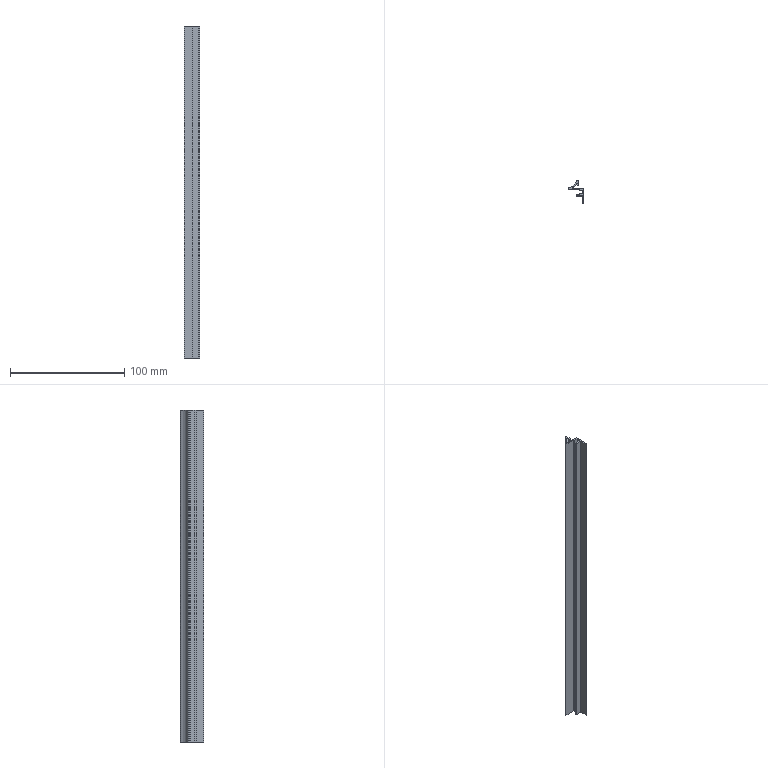Part | SolidWorks | features MoveFace 2, BaseBody 1, ICE 1 | 1 solid | 27 faces | box 14 x 20.3 x 291 mm | volume 14816 mm3 | plane 20 | cylinder 7 | commonest cylinder face diameters 0.387 x2 0.8 x2 0.4 x1 20 x1 22 x1
STEP:
#1=CARTESIAN_POINT('',(-5.304,-0.625,-867.));
#2=VERTEX_POINT('',#1);
#3=CARTESIAN_POINT('',(-5.449,-0.8125,-867.));
#4=VERTEX_POINT('',#3);
#5=CARTESIAN_POINT('',(-5.255,-0.8125,-867.));
#6=DIRECTION('',(0.,0.,1.));
#7=DIRECTION('',(-1.,0.,0.));
#8=AXIS2_PLACEMENT_3D('',#5,#6,#7);
#9=CIRCLE('',#8,0.1937);
#10=EDGE_CURVE('',#2,#4,#9,.T.);
#11=ORIENTED_EDGE('',*,*,#10,.T.);
#12=CARTESIAN_POINT('',(-5.449,-0.8125,-1158.));
#13=VERTEX_POINT('',#12);
#14=CARTESIAN_POINT('',(-5.449,-0.8125,230.));
#15=DIRECTION('',(0.,0.,-1.));
#16=VECTOR('',#15,1000.);
#17=LINE('',#14,#16);
#18=EDGE_CURVE('',#4,#13,#17,.T.);
#19=ORIENTED_EDGE('',*,*,#18,.T.);
#20=CARTESIAN_POINT('',(-5.304,-0.625,-1158.));
#21=VERTEX_POINT('',#20);
#22=CARTESIAN_POINT('',(-5.255,-0.8125,-1158.));
#23=DIRECTION('',(0.,0.,-1.));
#24=DIRECTION('',(1.,0.,0.));
#25=AXIS2_PLACEMENT_3D('',#22,#23,#24);
#26=CIRCLE('',#25,0.1937);
#27=EDGE_CURVE('',#13,#21,#26,.T.);
#28=ORIENTED_EDGE('',*,*,#27,.T.);
#29=CARTESIAN_POINT('',(-5.304,-0.625,230.));
#30=DIRECTION('',(0.,0.,-1.));
#31=VECTOR('',#30,1000.);
#32=LINE('',#29,#31);
#33=EDGE_CURVE('',#2,#21,#32,.T.);
#34=ORIENTED_EDGE('',*,*,#33,.F.);
#35=EDGE_LOOP('',(#11,#19,#28,#34));
#36=FACE_OUTER_BOUND('',#35,.T.);
#37=CARTESIAN_POINT('',(-5.255,-0.8125,230.));
#38=DIRECTION('',(0.,0.,-1.));
#39=DIRECTION('',(-1.,0.,0.));
#40=AXIS2_PLACEMENT_3D('',#37,#38,#39);
#41=CYLINDRICAL_SURFACE('',#40,0.1937);
#42=ADVANCED_FACE('',(#36),#41,.F.);
#43=CARTESIAN_POINT('',(5.,-1.,-1158.));
#44=VERTEX_POINT('',#43);
#45=CARTESIAN_POINT('',(5.,-14.3,-1158.));
#46=VERTEX_POINT('',#45);
#47=CARTESIAN_POINT('',(5.,29.623,-1158.));
#48=DIRECTION('',(0.,-1.,0.));
#49=VECTOR('',#48,1000.);
#50=LINE('',#47,#49);
#51=EDGE_CURVE('',#44,#46,#50,.T.);
#52=ORIENTED_EDGE('',*,*,#51,.F.);
#53=CARTESIAN_POINT('',(5.,-1.,-867.));
#54=VERTEX_POINT('',#53);
#55=CARTESIAN_POINT('',(5.,-1.,230.));
#56=DIRECTION('',(0.,0.,-1.));
#57=VECTOR('',#56,1000.);
#58=LINE('',#55,#57);
#59=EDGE_CURVE('',#54,#44,#58,.T.);
#60=ORIENTED_EDGE('',*,*,#59,.F.);
#61=CARTESIAN_POINT('',(5.,-14.3,-867.));
#62=VERTEX_POINT('',#61);
#63=CARTESIAN_POINT('',(5.,29.623,-867.));
#64=DIRECTION('',(0.,1.,0.));
#65=VECTOR('',#64,1000.);
#66=LINE('',#63,#65);
#67=EDGE_CURVE('',#62,#54,#66,.T.);
#68=ORIENTED_EDGE('',*,*,#67,.F.);
#69=CARTESIAN_POINT('',(5.,-14.3,230.));
#70=DIRECTION('',(0.,0.,1.));
#71=VECTOR('',#70,1000.);
#72=LINE('',#69,#71);
#73=EDGE_CURVE('',#46,#62,#72,.T.);
#74=ORIENTED_EDGE('',*,*,#73,.F.);
#75=EDGE_LOOP('',(#52,#60,#68,#74));
#76=FACE_OUTER_BOUND('',#75,.T.);
#77=CARTESIAN_POINT('',(5.,-14.3,230.));
#78=DIRECTION('',(-1.,0.,0.));
#79=DIRECTION('',(0.,0.,1.));
#80=AXIS2_PLACEMENT_3D('',#77,#78,#79);
#81=PLANE('',#80);
#82=ADVANCED_FACE('',(#76),#81,.F.);
#83=CARTESIAN_POINT('',(-9.,-2.,-1158.));
#84=VERTEX_POINT('',#83);
#85=CARTESIAN_POINT('',(-9.,-2.,-867.));
#86=VERTEX_POINT('',#85);
#87=CARTESIAN_POINT('',(-9.,-2.,230.));
#88=DIRECTION('',(0.,0.,1.));
#89=VECTOR('',#88,1000.);
#90=LINE('',#87,#89);
#91=EDGE_CURVE('',#84,#86,#90,.T.);
#92=ORIENTED_EDGE('',*,*,#91,.F.);
#93=CARTESIAN_POINT('',(0.9,-2.,-1158.));
#94=VERTEX_POINT('',#93);
#95=CARTESIAN_POINT('',(5.,-2.,-1158.));
#96=DIRECTION('',(-1.,0.,0.));
#97=VECTOR('',#96,1000.);
#98=LINE('',#95,#97);
#99=EDGE_CURVE('',#94,#84,#98,.T.);
#100=ORIENTED_EDGE('',*,*,#99,.F.);
#101=CARTESIAN_POINT('',(0.9,-2.,-867.));
#102=VERTEX_POINT('',#101);
#103=CARTESIAN_POINT('',(0.9,-2.,230.));
#104=DIRECTION('',(0.,0.,-1.));
#105=VECTOR('',#104,1000.);
#106=LINE('',#103,#105);
#107=EDGE_CURVE('',#102,#94,#106,.T.);
#108=ORIENTED_EDGE('',*,*,#107,.F.);
#109=CARTESIAN_POINT('',(5.,-2.,-867.));
#110=DIRECTION('',(1.,0.,0.));
#111=VECTOR('',#110,1000.);
#112=LINE('',#109,#111);
#113=EDGE_CURVE('',#86,#102,#112,.T.);
#114=ORIENTED_EDGE('',*,*,#113,.F.);
#115=EDGE_LOOP('',(#92,#100,#108,#114));
#116=FACE_OUTER_BOUND('',#115,.T.);
#117=CARTESIAN_POINT('',(-9.,-2.,230.));
#118=DIRECTION('',(0.,1.,0.));
#119=DIRECTION('',(0.,0.,1.));
#120=AXIS2_PLACEMENT_3D('',#117,#118,#119);
#121=PLANE('',#120);
#122=ADVANCED_FACE('',(#116),#121,.F.);
#123=CARTESIAN_POINT('',(4.,-6.,-867.));
#124=VERTEX_POINT('',#123);
#125=CARTESIAN_POINT('',(4.,-3.,-867.));
#126=VERTEX_POINT('',#125);
#127=CARTESIAN_POINT('',(4.,-3.,-867.));
#128=DIRECTION('',(0.,1.,0.));
#129=VECTOR('',#128,1000.);
#130=LINE('',#127,#129);
#131=EDGE_CURVE('',#124,#126,#130,.T.);
#132=ORIENTED_EDGE('',*,*,#131,.F.);
#133=CARTESIAN_POINT('',(1.,-6.,-867.));
#134=VERTEX_POINT('',#133);
#135=CARTESIAN_POINT('',(4.,-6.,-867.));
#136=DIRECTION('',(1.,0.,0.));
#137=VECTOR('',#136,1000.);
#138=LINE('',#135,#137);
#139=EDGE_CURVE('',#134,#124,#138,.T.);
#140=ORIENTED_EDGE('',*,*,#139,.F.);
#141=CARTESIAN_POINT('',(1.,-6.7,-867.));
#142=VERTEX_POINT('',#141);
#143=CARTESIAN_POINT('',(1.,29.623,-867.));
#144=DIRECTION('',(0.,-1.,0.));
#145=VECTOR('',#144,1000.);
#146=LINE('',#143,#145);
#147=EDGE_CURVE('',#134,#142,#146,.T.);
#148=ORIENTED_EDGE('',*,*,#147,.T.);
#149=CARTESIAN_POINT('',(-1.7,-6.7,-867.));
#150=VERTEX_POINT('',#149);
#151=CARTESIAN_POINT('',(1.,-6.7,-867.));
#152=DIRECTION('',(1.,0.,0.));
#153=VECTOR('',#152,1000.);
#154=LINE('',#151,#153);
#155=EDGE_CURVE('',#150,#142,#154,.T.);
#156=ORIENTED_EDGE('',*,*,#155,.F.);
#157=CARTESIAN_POINT('',(-1.7,-7.7,-867.));
#158=VERTEX_POINT('',#157);
#159=CARTESIAN_POINT('',(-1.7,29.623,-867.));
#160=DIRECTION('',(0.,-1.,0.));
#161=VECTOR('',#160,1000.);
#162=LINE('',#159,#161);
#163=EDGE_CURVE('',#150,#158,#162,.T.);
#164=ORIENTED_EDGE('',*,*,#163,.T.);
#165=CARTESIAN_POINT('',(4.,-7.7,-867.));
#166=VERTEX_POINT('',#165);
#167=CARTESIAN_POINT('',(-1.7,-7.7,-867.));
#168=DIRECTION('',(-1.,0.,0.));
#169=VECTOR('',#168,1000.);
#170=LINE('',#167,#169);
#171=EDGE_CURVE('',#166,#158,#170,.T.);
#172=ORIENTED_EDGE('',*,*,#171,.F.);
#173=CARTESIAN_POINT('',(4.,-14.3,-867.));
#174=VERTEX_POINT('',#173);
#175=CARTESIAN_POINT('',(4.,-7.7,-867.));
#176=DIRECTION('',(0.,1.,0.));
#177=VECTOR('',#176,1000.);
#178=LINE('',#175,#177);
#179=EDGE_CURVE('',#174,#166,#178,.T.);
#180=ORIENTED_EDGE('',*,*,#179,.F.);
#181=CARTESIAN_POINT('',(4.,-14.3,-867.));
#182=DIRECTION('',(-1.,0.,0.));
#183=VECTOR('',#182,1000.);
#184=LINE('',#181,#183);
#185=EDGE_CURVE('',#62,#174,#184,.T.);
#186=ORIENTED_EDGE('',*,*,#185,.F.);
#187=ORIENTED_EDGE('',*,*,#67,.T.);
#188=CARTESIAN_POINT('',(-5.207,-1.,-867.));
#189=VERTEX_POINT('',#188);
#190=CARTESIAN_POINT('',(5.,-1.,-867.));
#191=DIRECTION('',(1.,0.,0.));
#192=VECTOR('',#191,1000.);
#193=LINE('',#190,#192);
#194=EDGE_CURVE('',#189,#54,#193,.T.);
#195=ORIENTED_EDGE('',*,*,#194,.F.);
#196=CARTESIAN_POINT('',(-5.255,-0.8125,-867.));
#197=DIRECTION('',(0.,0.,1.));
#198=DIRECTION('',(-1.,0.,0.));
#199=AXIS2_PLACEMENT_3D('',#196,#197,#198);
#200=CIRCLE('',#199,0.1937);
#201=EDGE_CURVE('',#4,#189,#200,.T.);
#202=ORIENTED_EDGE('',*,*,#201,.F.);
#203=ORIENTED_EDGE('',*,*,#10,.F.);
#204=CARTESIAN_POINT('',(-1.368,3.063,-867.));
#205=VERTEX_POINT('',#204);
#206=CARTESIAN_POINT('',(-10.628,9.,-867.));
#207=DIRECTION('',(0.,0.,1.));
#208=DIRECTION('',(-1.,0.,0.));
#209=AXIS2_PLACEMENT_3D('',#206,#207,#208);
#210=CIRCLE('',#209,11.);
#211=EDGE_CURVE('',#2,#205,#210,.T.);
#212=ORIENTED_EDGE('',*,*,#211,.T.);
#213=CARTESIAN_POINT('',(-1.,2.955,-867.));
#214=VERTEX_POINT('',#213);
#215=CARTESIAN_POINT('',(-1.2,2.955,-867.));
#216=DIRECTION('',(0.,0.,1.));
#217=DIRECTION('',(-1.,0.,0.));
#218=AXIS2_PLACEMENT_3D('',#215,#216,#217);
#219=CIRCLE('',#218,0.2);
#220=EDGE_CURVE('',#214,#205,#219,.T.);
#221=ORIENTED_EDGE('',*,*,#220,.F.);
#222=CARTESIAN_POINT('',(-1.,1.5,-867.));
#223=VERTEX_POINT('',#222);
#224=CARTESIAN_POINT('',(-1.,2.955,-867.));
#225=DIRECTION('',(0.,1.,0.));
#226=VECTOR('',#225,1000.);
#227=LINE('',#224,#226);
#228=EDGE_CURVE('',#223,#214,#227,.T.);
#229=ORIENTED_EDGE('',*,*,#228,.F.);
#230=CARTESIAN_POINT('',(0.,1.5,-867.));
#231=VERTEX_POINT('',#230);
#232=CARTESIAN_POINT('',(-1.,1.5,-867.));
#233=DIRECTION('',(-1.,0.,0.));
#234=VECTOR('',#233,1000.);
#235=LINE('',#232,#234);
#236=EDGE_CURVE('',#231,#223,#235,.T.);
#237=ORIENTED_EDGE('',*,*,#236,.F.);
#238=CARTESIAN_POINT('',(0.,6.,-867.));
#239=VERTEX_POINT('',#238);
#240=CARTESIAN_POINT('',(0.,1.5,-867.));
#241=DIRECTION('',(0.,-1.,0.));
#242=VECTOR('',#241,1000.);
#243=LINE('',#240,#242);
#244=EDGE_CURVE('',#239,#231,#243,.T.);
#245=ORIENTED_EDGE('',*,*,#244,.F.);
#246=CARTESIAN_POINT('',(-0.8,6.,-867.));
#247=VERTEX_POINT('',#246);
#248=CARTESIAN_POINT('',(0.,6.,-867.));
#249=DIRECTION('',(1.,0.,0.));
#250=VECTOR('',#249,1000.);
#251=LINE('',#248,#250);
#252=EDGE_CURVE('',#247,#239,#251,.T.);
#253=ORIENTED_EDGE('',*,*,#252,.F.);
#254=CARTESIAN_POINT('',(-1.178,5.731,-867.));
#255=VERTEX_POINT('',#254);
#256=CARTESIAN_POINT('',(-0.8,5.6,-867.));
#257=DIRECTION('',(0.,0.,1.));
#258=DIRECTION('',(-1.,0.,0.));
#259=AXIS2_PLACEMENT_3D('',#256,#257,#258);
#260=CIRCLE('',#259,0.4);
#261=EDGE_CURVE('',#247,#255,#260,.T.);
#262=ORIENTED_EDGE('',*,*,#261,.T.);
#263=CARTESIAN_POINT('',(-8.678,-0.8077,-867.));
#264=VERTEX_POINT('',#263);
#265=CARTESIAN_POINT('',(-10.628,9.,-867.));
#266=DIRECTION('',(0.,0.,1.));
#267=DIRECTION('',(-1.,0.,0.));
#268=AXIS2_PLACEMENT_3D('',#265,#266,#267);
#269=CIRCLE('',#268,10.);
#270=EDGE_CURVE('',#264,#255,#269,.T.);
#271=ORIENTED_EDGE('',*,*,#270,.F.);
#272=CARTESIAN_POINT('',(-9.,-1.2,-867.));
#273=VERTEX_POINT('',#272);
#274=CARTESIAN_POINT('',(-8.6,-1.2,-867.));
#275=DIRECTION('',(0.,0.,1.));
#276=DIRECTION('',(-1.,0.,0.));
#277=AXIS2_PLACEMENT_3D('',#274,#275,#276);
#278=CIRCLE('',#277,0.4);
#279=EDGE_CURVE('',#264,#273,#278,.T.);
#280=ORIENTED_EDGE('',*,*,#279,.T.);
#281=CARTESIAN_POINT('',(-9.,29.623,-867.));
#282=DIRECTION('',(0.,-1.,0.));
#283=VECTOR('',#282,1000.);
#284=LINE('',#281,#283);
#285=EDGE_CURVE('',#273,#86,#284,.T.);
#286=ORIENTED_EDGE('',*,*,#285,.T.);
#287=ORIENTED_EDGE('',*,*,#113,.T.);
#288=CARTESIAN_POINT('',(0.9,-3.,-867.));
#289=VERTEX_POINT('',#288);
#290=CARTESIAN_POINT('',(0.9,-2.,-867.));
#291=DIRECTION('',(0.,1.,0.));
#292=VECTOR('',#291,1000.);
#293=LINE('',#290,#292);
#294=EDGE_CURVE('',#289,#102,#293,.T.);
#295=ORIENTED_EDGE('',*,*,#294,.F.);
#296=CARTESIAN_POINT('',(0.9,-3.,-867.));
#297=DIRECTION('',(-1.,0.,0.));
#298=VECTOR('',#297,1000.);
#299=LINE('',#296,#298);
#300=EDGE_CURVE('',#126,#289,#299,.T.);
#301=ORIENTED_EDGE('',*,*,#300,.F.);
#302=EDGE_LOOP('',(#132,#140,#148,#156,#164,#172,#180,#186,#187,#195,#202,#203,#212,#221,#229,#237,#245,#253,#262,#271,#280,#286,#287,#295,#301));
#303=FACE_OUTER_BOUND('',#302,.T.);
#304=CARTESIAN_POINT('',(5.,29.623,-867.));
#305=DIRECTION('',(0.,0.,-1.));
#306=DIRECTION('',(-1.,0.,0.));
#307=AXIS2_PLACEMENT_3D('',#304,#305,#306);
#308=PLANE('',#307);
#309=ADVANCED_FACE('',(#303),#308,.F.);
#310=ORIENTED_EDGE('',*,*,#185,.T.);
#311=CARTESIAN_POINT('',(4.,-14.3,-1158.));
#312=VERTEX_POINT('',#311);
#313=CARTESIAN_POINT('',(4.,-14.3,230.));
#314=DIRECTION('',(0.,0.,1.));
#315=VECTOR('',#314,1000.);
#316=LINE('',#313,#315);
#317=EDGE_CURVE('',#312,#174,#316,.T.);
#318=ORIENTED_EDGE('',*,*,#317,.F.);
#319=CARTESIAN_POINT('',(5.,-14.3,-1158.));
#320=DIRECTION('',(-1.,0.,0.));
#321=VECTOR('',#320,1000.);
#322=LINE('',#319,#321);
#323=EDGE_CURVE('',#46,#312,#322,.T.);
#324=ORIENTED_EDGE('',*,*,#323,.F.);
#325=ORIENTED_EDGE('',*,*,#73,.T.);
#326=EDGE_LOOP('',(#310,#318,#324,#325));
#327=FACE_OUTER_BOUND('',#326,.T.);
#328=CARTESIAN_POINT('',(4.,-14.3,230.));
#329=DIRECTION('',(0.,1.,0.));
#330=DIRECTION('',(0.,0.,1.));
#331=AXIS2_PLACEMENT_3D('',#328,#329,#330);
#332=PLANE('',#331);
#333=ADVANCED_FACE('',(#327),#332,.F.);
#334=ORIENTED_EDGE('',*,*,#51,.T.);
#335=ORIENTED_EDGE('',*,*,#323,.T.);
#336=CARTESIAN_POINT('',(4.,-7.7,-1158.));
#337=VERTEX_POINT('',#336);
#338=CARTESIAN_POINT('',(4.,-7.7,-1158.));
#339=DIRECTION('',(0.,-1.,0.));
#340=VECTOR('',#339,1000.);
#341=LINE('',#338,#340);
#342=EDGE_CURVE('',#337,#312,#341,.T.);
#343=ORIENTED_EDGE('',*,*,#342,.F.);
#344=CARTESIAN_POINT('',(-1.7,-7.7,-1158.));
#345=VERTEX_POINT('',#344);
#346=CARTESIAN_POINT('',(-1.7,-7.7,-1158.));
#347=DIRECTION('',(1.,0.,0.));
#348=VECTOR('',#347,1000.);
#349=LINE('',#346,#348);
#350=EDGE_CURVE('',#345,#337,#349,.T.);
#351=ORIENTED_EDGE('',*,*,#350,.F.);
#352=CARTESIAN_POINT('',(-1.7,-6.7,-1158.));
#353=VERTEX_POINT('',#352);
#354=CARTESIAN_POINT('',(-1.7,29.623,-1158.));
#355=DIRECTION('',(0.,1.,0.));
#356=VECTOR('',#355,1000.);
#357=LINE('',#354,#356);
#358=EDGE_CURVE('',#345,#353,#357,.T.);
#359=ORIENTED_EDGE('',*,*,#358,.T.);
#360=CARTESIAN_POINT('',(1.,-6.7,-1158.));
#361=VERTEX_POINT('',#360);
#362=CARTESIAN_POINT('',(1.,-6.7,-1158.));
#363=DIRECTION('',(-1.,0.,0.));
#364=VECTOR('',#363,1000.);
#365=LINE('',#362,#364);
#366=EDGE_CURVE('',#361,#353,#365,.T.);
#367=ORIENTED_EDGE('',*,*,#366,.F.);
#368=CARTESIAN_POINT('',(1.,-6.,-1158.));
#369=VERTEX_POINT('',#368);
#370=CARTESIAN_POINT('',(1.,29.623,-1158.));
#371=DIRECTION('',(0.,1.,0.));
#372=VECTOR('',#371,1000.);
#373=LINE('',#370,#372);
#374=EDGE_CURVE('',#361,#369,#373,.T.);
#375=ORIENTED_EDGE('',*,*,#374,.T.);
#376=CARTESIAN_POINT('',(4.,-6.,-1158.));
#377=VERTEX_POINT('',#376);
#378=CARTESIAN_POINT('',(4.,-6.,-1158.));
#379=DIRECTION('',(-1.,0.,0.));
#380=VECTOR('',#379,1000.);
#381=LINE('',#378,#380);
#382=EDGE_CURVE('',#377,#369,#381,.T.);
#383=ORIENTED_EDGE('',*,*,#382,.F.);
#384=CARTESIAN_POINT('',(4.,-3.,-1158.));
#385=VERTEX_POINT('',#384);
#386=CARTESIAN_POINT('',(4.,-3.,-1158.));
#387=DIRECTION('',(0.,-1.,0.));
#388=VECTOR('',#387,1000.);
#389=LINE('',#386,#388);
#390=EDGE_CURVE('',#385,#377,#389,.T.);
#391=ORIENTED_EDGE('',*,*,#390,.F.);
#392=CARTESIAN_POINT('',(0.9,-3.,-1158.));
#393=VERTEX_POINT('',#392);
#394=CARTESIAN_POINT('',(0.9,-3.,-1158.));
#395=DIRECTION('',(1.,0.,0.));
#396=VECTOR('',#395,1000.);
#397=LINE('',#394,#396);
#398=EDGE_CURVE('',#393,#385,#397,.T.);
#399=ORIENTED_EDGE('',*,*,#398,.F.);
#400=CARTESIAN_POINT('',(0.9,-2.,-1158.));
#401=DIRECTION('',(0.,-1.,0.));
#402=VECTOR('',#401,1000.);
#403=LINE('',#400,#402);
#404=EDGE_CURVE('',#94,#393,#403,.T.);
#405=ORIENTED_EDGE('',*,*,#404,.F.);
#406=ORIENTED_EDGE('',*,*,#99,.T.);
#407=CARTESIAN_POINT('',(-9.,-1.2,-1158.));
#408=VERTEX_POINT('',#407);
#409=CARTESIAN_POINT('',(-9.,-1.2,-1158.));
#410=DIRECTION('',(0.,-1.,0.));
#411=VECTOR('',#410,1000.);
#412=LINE('',#409,#411);
#413=EDGE_CURVE('',#408,#84,#412,.T.);
#414=ORIENTED_EDGE('',*,*,#413,.F.);
#415=CARTESIAN_POINT('',(-8.678,-0.8077,-1158.));
#416=VERTEX_POINT('',#415);
#417=CARTESIAN_POINT('',(-8.6,-1.2,-1158.));
#418=DIRECTION('',(0.,0.,-1.));
#419=DIRECTION('',(1.,0.,0.));
#420=AXIS2_PLACEMENT_3D('',#417,#418,#419);
#421=CIRCLE('',#420,0.4);
#422=EDGE_CURVE('',#408,#416,#421,.T.);
#423=ORIENTED_EDGE('',*,*,#422,.T.);
#424=CARTESIAN_POINT('',(-1.178,5.731,-1158.));
#425=VERTEX_POINT('',#424);
#426=CARTESIAN_POINT('',(-10.628,9.,-1158.));
#427=DIRECTION('',(0.,0.,-1.));
#428=DIRECTION('',(1.,0.,0.));
#429=AXIS2_PLACEMENT_3D('',#426,#427,#428);
#430=CIRCLE('',#429,10.);
#431=EDGE_CURVE('',#425,#416,#430,.T.);
#432=ORIENTED_EDGE('',*,*,#431,.F.);
#433=CARTESIAN_POINT('',(-0.8,6.,-1158.));
#434=VERTEX_POINT('',#433);
#435=CARTESIAN_POINT('',(-0.8,5.6,-1158.));
#436=DIRECTION('',(0.,0.,-1.));
#437=DIRECTION('',(1.,0.,0.));
#438=AXIS2_PLACEMENT_3D('',#435,#436,#437);
#439=CIRCLE('',#438,0.4);
#440=EDGE_CURVE('',#425,#434,#439,.T.);
#441=ORIENTED_EDGE('',*,*,#440,.T.);
#442=CARTESIAN_POINT('',(0.,6.,-1158.));
#443=VERTEX_POINT('',#442);
#444=CARTESIAN_POINT('',(0.,6.,-1158.));
#445=DIRECTION('',(-1.,0.,0.));
#446=VECTOR('',#445,1000.);
#447=LINE('',#444,#446);
#448=EDGE_CURVE('',#443,#434,#447,.T.);
#449=ORIENTED_EDGE('',*,*,#448,.F.);
#450=CARTESIAN_POINT('',(0.,1.5,-1158.));
#451=VERTEX_POINT('',#450);
#452=CARTESIAN_POINT('',(0.,1.5,-1158.));
#453=DIRECTION('',(0.,1.,0.));
#454=VECTOR('',#453,1000.);
#455=LINE('',#452,#454);
#456=EDGE_CURVE('',#451,#443,#455,.T.);
#457=ORIENTED_EDGE('',*,*,#456,.F.);
#458=CARTESIAN_POINT('',(-1.,1.5,-1158.));
#459=VERTEX_POINT('',#458);
#460=CARTESIAN_POINT('',(-1.,1.5,-1158.));
#461=DIRECTION('',(1.,0.,0.));
#462=VECTOR('',#461,1000.);
#463=LINE('',#460,#462);
#464=EDGE_CURVE('',#459,#451,#463,.T.);
#465=ORIENTED_EDGE('',*,*,#464,.F.);
#466=CARTESIAN_POINT('',(-1.,2.955,-1158.));
#467=VERTEX_POINT('',#466);
#468=CARTESIAN_POINT('',(-1.,2.955,-1158.));
#469=DIRECTION('',(0.,-1.,0.));
#470=VECTOR('',#469,1000.);
#471=LINE('',#468,#470);
#472=EDGE_CURVE('',#467,#459,#471,.T.);
#473=ORIENTED_EDGE('',*,*,#472,.F.);
#474=CARTESIAN_POINT('',(-1.368,3.063,-1158.));
#475=VERTEX_POINT('',#474);
#476=CARTESIAN_POINT('',(-1.2,2.955,-1158.));
#477=DIRECTION('',(0.,0.,-1.));
#478=DIRECTION('',(1.,0.,0.));
#479=AXIS2_PLACEMENT_3D('',#476,#477,#478);
#480=CIRCLE('',#479,0.2);
#481=EDGE_CURVE('',#475,#467,#480,.T.);
#482=ORIENTED_EDGE('',*,*,#481,.F.);
#483=CARTESIAN_POINT('',(-10.628,9.,-1158.));
#484=DIRECTION('',(0.,0.,-1.));
#485=DIRECTION('',(1.,0.,0.));
#486=AXIS2_PLACEMENT_3D('',#483,#484,#485);
#487=CIRCLE('',#486,11.);
#488=EDGE_CURVE('',#475,#21,#487,.T.);
#489=ORIENTED_EDGE('',*,*,#488,.T.);
#490=ORIENTED_EDGE('',*,*,#27,.F.);
#491=CARTESIAN_POINT('',(-5.207,-1.,-1158.));
#492=VERTEX_POINT('',#491);
#493=CARTESIAN_POINT('',(-5.255,-0.8125,-1158.));
#494=DIRECTION('',(0.,0.,-1.));
#495=DIRECTION('',(1.,0.,0.));
#496=AXIS2_PLACEMENT_3D('',#493,#494,#495);
#497=CIRCLE('',#496,0.1937);
#498=EDGE_CURVE('',#492,#13,#497,.T.);
#499=ORIENTED_EDGE('',*,*,#498,.F.);
#500=CARTESIAN_POINT('',(5.,-1.,-1158.));
#501=DIRECTION('',(-1.,0.,0.));
#502=VECTOR('',#501,1000.);
#503=LINE('',#500,#502);
#504=EDGE_CURVE('',#44,#492,#503,.T.);
#505=ORIENTED_EDGE('',*,*,#504,.F.);
#506=EDGE_LOOP('',(#334,#335,#343,#351,#359,#367,#375,#383,#391,#399,#405,#406,#414,#423,#432,#441,#449,#457,#465,#473,#482,#489,#490,#499,#505));
#507=FACE_OUTER_BOUND('',#506,.T.);
#508=CARTESIAN_POINT('',(5.,29.623,-1158.));
#509=DIRECTION('',(0.,0.,1.));
#510=DIRECTION('',(1.,0.,0.));
#511=AXIS2_PLACEMENT_3D('',#508,#509,#510);
#512=PLANE('',#511);
#513=ADVANCED_FACE('',(#507),#512,.F.);
#514=ORIENTED_EDGE('',*,*,#59,.T.);
#515=ORIENTED_EDGE('',*,*,#504,.T.);
#516=CARTESIAN_POINT('',(-5.207,-1.,230.));
#517=DIRECTION('',(0.,0.,-1.));
#518=VECTOR('',#517,1000.);
#519=LINE('',#516,#518);
#520=EDGE_CURVE('',#189,#492,#519,.T.);
#521=ORIENTED_EDGE('',*,*,#520,.F.);
#522=ORIENTED_EDGE('',*,*,#194,.T.);
#523=EDGE_LOOP('',(#514,#515,#521,#522));
#524=FACE_OUTER_BOUND('',#523,.T.);
#525=CARTESIAN_POINT('',(5.,-1.,230.));
#526=DIRECTION('',(0.,-1.,0.));
#527=DIRECTION('',(0.,0.,-1.));
#528=AXIS2_PLACEMENT_3D('',#525,#526,#527);
#529=PLANE('',#528);
#530=ADVANCED_FACE('',(#524),#529,.F.);
#531=CARTESIAN_POINT('',(-9.,-1.2,230.));
#532=DIRECTION('',(0.,0.,1.));
#533=VECTOR('',#532,1000.);
#534=LINE('',#531,#533);
#535=EDGE_CURVE('',#408,#273,#534,.T.);
#536=ORIENTED_EDGE('',*,*,#535,.F.);
#537=ORIENTED_EDGE('',*,*,#413,.T.);
#538=ORIENTED_EDGE('',*,*,#91,.T.);
#539=ORIENTED_EDGE('',*,*,#285,.F.);
#540=EDGE_LOOP('',(#536,#537,#538,#539));
#541=FACE_OUTER_BOUND('',#540,.T.);
#542=CARTESIAN_POINT('',(-9.,-1.2,230.));
#543=DIRECTION('',(1.,0.,0.));
#544=DIRECTION('',(0.,0.,-1.));
#545=AXIS2_PLACEMENT_3D('',#542,#543,#544);
#546=PLANE('',#545);
#547=ADVANCED_FACE('',(#541),#546,.F.);
#548=ORIENTED_EDGE('',*,*,#294,.T.);
#549=ORIENTED_EDGE('',*,*,#107,.T.);
#550=ORIENTED_EDGE('',*,*,#404,.T.);
#551=CARTESIAN_POINT('',(0.9,-3.,230.));
#552=DIRECTION('',(0.,0.,-1.));
#553=VECTOR('',#552,1000.);
#554=LINE('',#551,#553);
#555=EDGE_CURVE('',#289,#393,#554,.T.);
#556=ORIENTED_EDGE('',*,*,#555,.F.);
#557=EDGE_LOOP('',(#548,#549,#550,#556));
#558=FACE_OUTER_BOUND('',#557,.T.);
#559=CARTESIAN_POINT('',(0.9,-2.,230.));
#560=DIRECTION('',(1.,0.,0.));
#561=DIRECTION('',(0.,0.,-1.));
#562=AXIS2_PLACEMENT_3D('',#559,#560,#561);
#563=PLANE('',#562);
#564=ADVANCED_FACE('',(#558),#563,.F.);
#565=ORIENTED_EDGE('',*,*,#300,.T.);
#566=ORIENTED_EDGE('',*,*,#555,.T.);
#567=ORIENTED_EDGE('',*,*,#398,.T.);
#568=CARTESIAN_POINT('',(4.,-3.,230.));
#569=DIRECTION('',(0.,0.,-1.));
#570=VECTOR('',#569,1000.);
#571=LINE('',#568,#570);
#572=EDGE_CURVE('',#126,#385,#571,.T.);
#573=ORIENTED_EDGE('',*,*,#572,.F.);
#574=EDGE_LOOP('',(#565,#566,#567,#573));
#575=FACE_OUTER_BOUND('',#574,.T.);
#576=CARTESIAN_POINT('',(0.9,-3.,230.));
#577=DIRECTION('',(0.,1.,0.));
#578=DIRECTION('',(0.,0.,1.));
#579=AXIS2_PLACEMENT_3D('',#576,#577,#578);
#580=PLANE('',#579);
#581=ADVANCED_FACE('',(#575),#580,.F.);
#582=ORIENTED_EDGE('',*,*,#131,.T.);
#583=ORIENTED_EDGE('',*,*,#572,.T.);
#584=ORIENTED_EDGE('',*,*,#390,.T.);
#585=CARTESIAN_POINT('',(4.,-6.,230.));
#586=DIRECTION('',(0.,0.,-1.));
#587=VECTOR('',#586,1000.);
#588=LINE('',#585,#587);
#589=EDGE_CURVE('',#124,#377,#588,.T.);
#590=ORIENTED_EDGE('',*,*,#589,.F.);
#591=EDGE_LOOP('',(#582,#583,#584,#590));
#592=FACE_OUTER_BOUND('',#591,.T.);
#593=CARTESIAN_POINT('',(4.,-3.,230.));
#594=DIRECTION('',(1.,0.,0.));
#595=DIRECTION('',(0.,0.,-1.));
#596=AXIS2_PLACEMENT_3D('',#593,#594,#595);
#597=PLANE('',#596);
#598=ADVANCED_FACE('',(#592),#597,.F.);
#599=ORIENTED_EDGE('',*,*,#139,.T.);
#600=ORIENTED_EDGE('',*,*,#589,.T.);
#601=ORIENTED_EDGE('',*,*,#382,.T.);
#602=CARTESIAN_POINT('',(1.,-6.,230.));
#603=DIRECTION('',(0.,0.,-1.));
#604=VECTOR('',#603,1000.);
#605=LINE('',#602,#604);
#606=EDGE_CURVE('',#134,#369,#605,.T.);
#607=ORIENTED_EDGE('',*,*,#606,.F.);
#608=EDGE_LOOP('',(#599,#600,#601,#607));
#609=FACE_OUTER_BOUND('',#608,.T.);
#610=CARTESIAN_POINT('',(4.,-6.,230.));
#611=DIRECTION('',(0.,-1.,0.));
#612=DIRECTION('',(0.,0.,-1.));
#613=AXIS2_PLACEMENT_3D('',#610,#611,#612);
#614=PLANE('',#613);
#615=ADVANCED_FACE('',(#609),#614,.F.);
#616=ORIENTED_EDGE('',*,*,#155,.T.);
#617=CARTESIAN_POINT('',(1.,-6.7,230.));
#618=DIRECTION('',(0.,0.,1.));
#619=VECTOR('',#618,1000.);
#620=LINE('',#617,#619);
#621=EDGE_CURVE('',#361,#142,#620,.T.);
#622=ORIENTED_EDGE('',*,*,#621,.F.);
#623=ORIENTED_EDGE('',*,*,#366,.T.);
#624=CARTESIAN_POINT('',(-1.7,-6.7,230.));
#625=DIRECTION('',(0.,0.,-1.));
#626=VECTOR('',#625,1000.);
#627=LINE('',#624,#626);
#628=EDGE_CURVE('',#150,#353,#627,.T.);
#629=ORIENTED_EDGE('',*,*,#628,.F.);
#630=EDGE_LOOP('',(#616,#622,#623,#629));
#631=FACE_OUTER_BOUND('',#630,.T.);
#632=CARTESIAN_POINT('',(1.,-6.7,230.));
#633=DIRECTION('',(0.,-1.,0.));
#634=DIRECTION('',(0.,0.,-1.));
#635=AXIS2_PLACEMENT_3D('',#632,#633,#634);
#636=PLANE('',#635);
#637=ADVANCED_FACE('',(#631),#636,.F.);
#638=ORIENTED_EDGE('',*,*,#171,.T.);
#639=CARTESIAN_POINT('',(-1.7,-7.7,230.));
#640=DIRECTION('',(0.,0.,1.));
#641=VECTOR('',#640,1000.);
#642=LINE('',#639,#641);
#643=EDGE_CURVE('',#345,#158,#642,.T.);
#644=ORIENTED_EDGE('',*,*,#643,.F.);
#645=ORIENTED_EDGE('',*,*,#350,.T.);
#646=CARTESIAN_POINT('',(4.,-7.7,230.));
#647=DIRECTION('',(0.,0.,-1.));
#648=VECTOR('',#647,1000.);
#649=LINE('',#646,#648);
#650=EDGE_CURVE('',#166,#337,#649,.T.);
#651=ORIENTED_EDGE('',*,*,#650,.F.);
#652=EDGE_LOOP('',(#638,#644,#645,#651));
#653=FACE_OUTER_BOUND('',#652,.T.);
#654=CARTESIAN_POINT('',(-1.7,-7.7,230.));
#655=DIRECTION('',(0.,1.,0.));
#656=DIRECTION('',(0.,0.,1.));
#657=AXIS2_PLACEMENT_3D('',#654,#655,#656);
#658=PLANE('',#657);
#659=ADVANCED_FACE('',(#653),#658,.F.);
#660=ORIENTED_EDGE('',*,*,#179,.T.);
#661=ORIENTED_EDGE('',*,*,#650,.T.);
#662=ORIENTED_EDGE('',*,*,#342,.T.);
#663=ORIENTED_EDGE('',*,*,#317,.T.);
#664=EDGE_LOOP('',(#660,#661,#662,#663));
#665=FACE_OUTER_BOUND('',#664,.T.);
#666=CARTESIAN_POINT('',(4.,-7.7,230.));
#667=DIRECTION('',(1.,0.,0.));
#668=DIRECTION('',(0.,0.,-1.));
#669=AXIS2_PLACEMENT_3D('',#666,#667,#668);
#670=PLANE('',#669);
#671=ADVANCED_FACE('',(#665),#670,.F.);
#672=ORIENTED_EDGE('',*,*,#18,.F.);
#673=ORIENTED_EDGE('',*,*,#201,.T.);
#674=ORIENTED_EDGE('',*,*,#520,.T.);
#675=ORIENTED_EDGE('',*,*,#498,.T.);
#676=EDGE_LOOP('',(#672,#673,#674,#675));
#677=FACE_OUTER_BOUND('',#676,.T.);
#678=CARTESIAN_POINT('',(-5.255,-0.8125,230.));
#679=DIRECTION('',(0.,0.,-1.));
#680=DIRECTION('',(-1.,0.,0.));
#681=AXIS2_PLACEMENT_3D('',#678,#679,#680);
#682=CYLINDRICAL_SURFACE('',#681,0.1937);
#683=ADVANCED_FACE('',(#677),#682,.F.);
#684=CARTESIAN_POINT('',(-1.,2.955,230.));
#685=DIRECTION('',(0.,0.,1.));
#686=VECTOR('',#685,1000.);
#687=LINE('',#684,#686);
#688=EDGE_CURVE('',#467,#214,#687,.T.);
#689=ORIENTED_EDGE('',*,*,#688,.F.);
#690=ORIENTED_EDGE('',*,*,#472,.T.);
#691=CARTESIAN_POINT('',(-1.,1.5,230.));
#692=DIRECTION('',(0.,0.,-1.));
#693=VECTOR('',#692,1000.);
#694=LINE('',#691,#693);
#695=EDGE_CURVE('',#223,#459,#694,.T.);
#696=ORIENTED_EDGE('',*,*,#695,.F.);
#697=ORIENTED_EDGE('',*,*,#228,.T.);
#698=EDGE_LOOP('',(#689,#690,#696,#697));
#699=FACE_OUTER_BOUND('',#698,.T.);
#700=CARTESIAN_POINT('',(-1.,2.955,230.));
#701=DIRECTION('',(1.,0.,0.));
#702=DIRECTION('',(0.,0.,-1.));
#703=AXIS2_PLACEMENT_3D('',#700,#701,#702);
#704=PLANE('',#703);
#705=ADVANCED_FACE('',(#699),#704,.F.);
#706=ORIENTED_EDGE('',*,*,#488,.F.);
#707=CARTESIAN_POINT('',(-1.368,3.063,230.));
#708=DIRECTION('',(0.,0.,1.));
#709=VECTOR('',#708,1000.);
#710=LINE('',#707,#709);
#711=EDGE_CURVE('',#475,#205,#710,.T.);
#712=ORIENTED_EDGE('',*,*,#711,.T.);
#713=ORIENTED_EDGE('',*,*,#211,.F.);
#714=ORIENTED_EDGE('',*,*,#33,.T.);
#715=EDGE_LOOP('',(#706,#712,#713,#714));
#716=FACE_OUTER_BOUND('',#715,.T.);
#717=CARTESIAN_POINT('',(-10.628,9.,230.));
#718=DIRECTION('',(0.,0.,-1.));
#719=DIRECTION('',(-1.,0.,0.));
#720=AXIS2_PLACEMENT_3D('',#717,#718,#719);
#721=CYLINDRICAL_SURFACE('',#720,11.);
#722=ADVANCED_FACE('',(#716),#721,.T.);
#723=CARTESIAN_POINT('',(-1.178,5.731,230.));
#724=DIRECTION('',(0.,0.,1.));
#725=VECTOR('',#724,1000.);
#726=LINE('',#723,#725);
#727=EDGE_CURVE('',#425,#255,#726,.T.);
#728=ORIENTED_EDGE('',*,*,#727,.F.);
#729=ORIENTED_EDGE('',*,*,#431,.T.);
#730=CARTESIAN_POINT('',(-8.678,-0.8077,230.));
#731=DIRECTION('',(0.,0.,-1.));
#732=VECTOR('',#731,1000.);
#733=LINE('',#730,#732);
#734=EDGE_CURVE('',#264,#416,#733,.T.);
#735=ORIENTED_EDGE('',*,*,#734,.F.);
#736=ORIENTED_EDGE('',*,*,#270,.T.);
#737=EDGE_LOOP('',(#728,#729,#735,#736));
#738=FACE_OUTER_BOUND('',#737,.T.);
#739=CARTESIAN_POINT('',(-10.628,9.,230.));
#740=DIRECTION('',(0.,0.,-1.));
#741=DIRECTION('',(-1.,0.,0.));
#742=AXIS2_PLACEMENT_3D('',#739,#740,#741);
#743=CYLINDRICAL_SURFACE('',#742,10.);
#744=ADVANCED_FACE('',(#738),#743,.F.);
#745=CARTESIAN_POINT('',(0.,1.5,230.));
#746=DIRECTION('',(0.,0.,1.));
#747=VECTOR('',#746,1000.);
#748=LINE('',#745,#747);
#749=EDGE_CURVE('',#451,#231,#748,.T.);
#750=ORIENTED_EDGE('',*,*,#749,.F.);
#751=ORIENTED_EDGE('',*,*,#456,.T.);
#752=CARTESIAN_POINT('',(0.,6.,230.));
#753=DIRECTION('',(0.,0.,-1.));
#754=VECTOR('',#753,1000.);
#755=LINE('',#752,#754);
#756=EDGE_CURVE('',#239,#443,#755,.T.);
#757=ORIENTED_EDGE('',*,*,#756,.F.);
#758=ORIENTED_EDGE('',*,*,#244,.T.);
#759=EDGE_LOOP('',(#750,#751,#757,#758));
#760=FACE_OUTER_BOUND('',#759,.T.);
#761=CARTESIAN_POINT('',(0.,1.5,230.));
#762=DIRECTION('',(-1.,0.,0.));
#763=DIRECTION('',(0.,0.,1.));
#764=AXIS2_PLACEMENT_3D('',#761,#762,#763);
#765=PLANE('',#764);
#766=ADVANCED_FACE('',(#760),#765,.F.);
#767=ORIENTED_EDGE('',*,*,#422,.F.);
#768=ORIENTED_EDGE('',*,*,#535,.T.);
#769=ORIENTED_EDGE('',*,*,#279,.F.);
#770=ORIENTED_EDGE('',*,*,#734,.T.);
#771=EDGE_LOOP('',(#767,#768,#769,#770));
#772=FACE_OUTER_BOUND('',#771,.T.);
#773=CARTESIAN_POINT('',(-8.6,-1.2,230.));
#774=DIRECTION('',(0.,0.,-1.));
#775=DIRECTION('',(-1.,0.,0.));
#776=AXIS2_PLACEMENT_3D('',#773,#774,#775);
#777=CYLINDRICAL_SURFACE('',#776,0.4);
#778=ADVANCED_FACE('',(#772),#777,.T.);
#779=ORIENTED_EDGE('',*,*,#147,.F.);
#780=ORIENTED_EDGE('',*,*,#606,.T.);
#781=ORIENTED_EDGE('',*,*,#374,.F.);
#782=ORIENTED_EDGE('',*,*,#621,.T.);
#783=EDGE_LOOP('',(#779,#780,#781,#782));
#784=FACE_OUTER_BOUND('',#783,.T.);
#785=CARTESIAN_POINT('',(1.,-6.,230.));
#786=DIRECTION('',(1.,0.,0.));
#787=DIRECTION('',(0.,0.,-1.));
#788=AXIS2_PLACEMENT_3D('',#785,#786,#787);
#789=PLANE('',#788);
#790=ADVANCED_FACE('',(#784),#789,.F.);
#791=ORIENTED_EDGE('',*,*,#163,.F.);
#792=ORIENTED_EDGE('',*,*,#628,.T.);
#793=ORIENTED_EDGE('',*,*,#358,.F.);
#794=ORIENTED_EDGE('',*,*,#643,.T.);
#795=EDGE_LOOP('',(#791,#792,#793,#794));
#796=FACE_OUTER_BOUND('',#795,.T.);
#797=CARTESIAN_POINT('',(-1.7,-6.7,230.));
#798=DIRECTION('',(1.,0.,0.));
#799=DIRECTION('',(0.,0.,-1.));
#800=AXIS2_PLACEMENT_3D('',#797,#798,#799);
#801=PLANE('',#800);
#802=ADVANCED_FACE('',(#796),#801,.F.);
#803=ORIENTED_EDGE('',*,*,#711,.F.);
#804=ORIENTED_EDGE('',*,*,#481,.T.);
#805=ORIENTED_EDGE('',*,*,#688,.T.);
#806=ORIENTED_EDGE('',*,*,#220,.T.);
#807=EDGE_LOOP('',(#803,#804,#805,#806));
#808=FACE_OUTER_BOUND('',#807,.T.);
#809=CARTESIAN_POINT('',(-1.2,2.955,230.));
#810=DIRECTION('',(0.,0.,-1.));
#811=DIRECTION('',(-1.,0.,0.));
#812=AXIS2_PLACEMENT_3D('',#809,#810,#811);
#813=CYLINDRICAL_SURFACE('',#812,0.2);
#814=ADVANCED_FACE('',(#808),#813,.F.);
#815=ORIENTED_EDGE('',*,*,#695,.T.);
#816=ORIENTED_EDGE('',*,*,#464,.T.);
#817=ORIENTED_EDGE('',*,*,#749,.T.);
#818=ORIENTED_EDGE('',*,*,#236,.T.);
#819=EDGE_LOOP('',(#815,#816,#817,#818));
#820=FACE_OUTER_BOUND('',#819,.T.);
#821=CARTESIAN_POINT('',(-1.,1.5,230.));
#822=DIRECTION('',(0.,1.,0.));
#823=DIRECTION('',(0.,0.,1.));
#824=AXIS2_PLACEMENT_3D('',#821,#822,#823);
#825=PLANE('',#824);
#826=ADVANCED_FACE('',(#820),#825,.F.);
#827=ORIENTED_EDGE('',*,*,#440,.F.);
#828=ORIENTED_EDGE('',*,*,#727,.T.);
#829=ORIENTED_EDGE('',*,*,#261,.F.);
#830=CARTESIAN_POINT('',(-0.8,6.,230.));
#831=DIRECTION('',(0.,0.,-1.));
#832=VECTOR('',#831,1000.);
#833=LINE('',#830,#832);
#834=EDGE_CURVE('',#247,#434,#833,.T.);
#835=ORIENTED_EDGE('',*,*,#834,.T.);
#836=EDGE_LOOP('',(#827,#828,#829,#835));
#837=FACE_OUTER_BOUND('',#836,.T.);
#838=CARTESIAN_POINT('',(-0.8,5.6,230.));
#839=DIRECTION('',(0.,0.,-1.));
#840=DIRECTION('',(-1.,0.,0.));
#841=AXIS2_PLACEMENT_3D('',#838,#839,#840);
#842=CYLINDRICAL_SURFACE('',#841,0.4);
#843=ADVANCED_FACE('',(#837),#842,.T.);
#844=ORIENTED_EDGE('',*,*,#756,.T.);
#845=ORIENTED_EDGE('',*,*,#448,.T.);
#846=ORIENTED_EDGE('',*,*,#834,.F.);
#847=ORIENTED_EDGE('',*,*,#252,.T.);
#848=EDGE_LOOP('',(#844,#845,#846,#847));
#849=FACE_OUTER_BOUND('',#848,.T.);
#850=CARTESIAN_POINT('',(0.,6.,230.));
#851=DIRECTION('',(0.,-1.,0.));
#852=DIRECTION('',(0.,0.,-1.));
#853=AXIS2_PLACEMENT_3D('',#850,#851,#852);
#854=PLANE('',#853);
#855=ADVANCED_FACE('',(#849),#854,.F.);
#856=CLOSED_SHELL('',(#42,#82,#122,#309,#333,#513,#530,#547,#564,#581,#598,#615,#637,#659,#671,#683,#705,#722,#744,#766,#778,#790,#802,#814,#826,#843,#855));
#857=MANIFOLD_SOLID_BREP('',#856);
#858=CARTESIAN_POINT('',(0.,0.,0.));
#859=DIRECTION('',(0.,0.,1.));
#860=DIRECTION('',(1.,0.,0.));
#861=AXIS2_PLACEMENT_3D('',#858,#859,#860);
#862=(LENGTH_UNIT()NAMED_UNIT(*)SI_UNIT(.MILLI.,.METRE.));
#863=UNCERTAINTY_MEASURE_WITH_UNIT(LENGTH_MEASURE(0.00001),#862,'','');
#864=(NAMED_UNIT(*)PLANE_ANGLE_UNIT()SI_UNIT($,.RADIAN.));
#865=(NAMED_UNIT(*)SI_UNIT($,.STERADIAN.)SOLID_ANGLE_UNIT());
#866=(GEOMETRIC_REPRESENTATION_CONTEXT(3)GLOBAL_UNCERTAINTY_ASSIGNED_CONTEXT((#863))GLOBAL_UNIT_ASSIGNED_CONTEXT((#862,#864,#865))REPRESENTATION_CONTEXT('',''));
#867=ADVANCED_BREP_SHAPE_REPRESENTATION('',(#857,#861),#866);